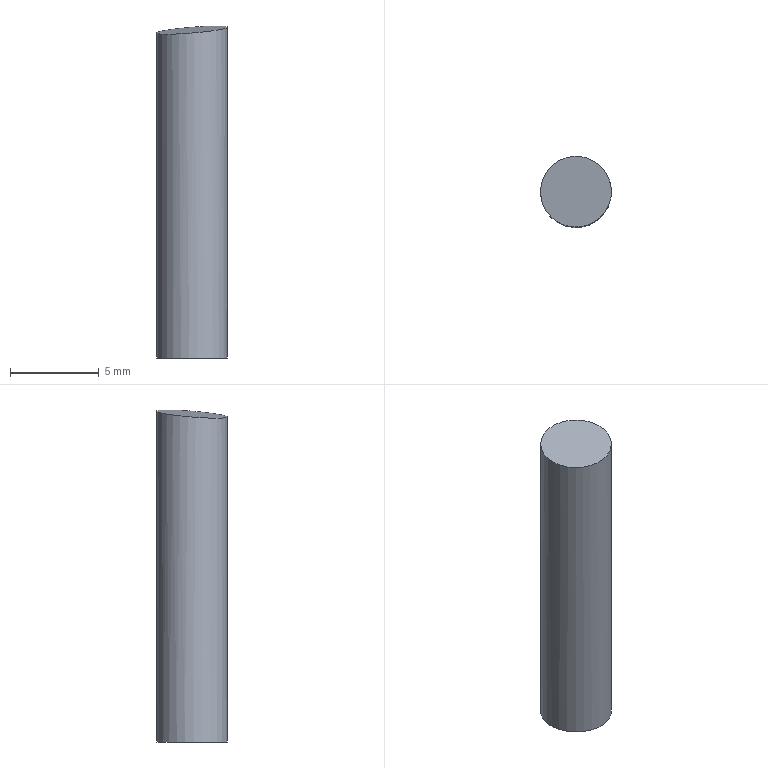Part | NX | features solid 2 | 1 solid | 3 faces | box 4 x 4 x 18.751 mm | volume 232.708 mm3 | plane 2 | cylinder 1 | commonest cylinder face diameters 4 x1
STEP:
#1=CARTESIAN_POINT('',(660.583,-7.761,-27.));
#2=VERTEX_POINT('',#1);
#3=CARTESIAN_POINT('',(658.583,-7.761,-27.));
#4=DIRECTION('',(0.,0.,1.));
#5=DIRECTION('',(1.,0.,0.));
#6=AXIS2_PLACEMENT_3D('',#3,#4,#5);
#7=CIRCLE('',#6,2.);
#8=EDGE_CURVE('',#2,#2,#7,.T.);
#9=ORIENTED_EDGE('',*,*,#8,.F.);
#10=EDGE_LOOP('',(#9));
#11=FACE_BOUND('',#10,.T.);
#12=CARTESIAN_POINT('',(658.583,-7.761,-27.));
#13=DIRECTION('',(0.,0.,-1.));
#14=DIRECTION('',(-1.,0.,0.));
#15=AXIS2_PLACEMENT_3D('',#12,#13,#14);
#16=PLANE('',#15);
#17=ADVANCED_FACE('',(#11),#16,.T.);
#18=CARTESIAN_POINT('',(657.162,-9.168,-8.714));
#19=VERTEX_POINT('',#18);
#20=CARTESIAN_POINT('',(658.583,-7.761,-8.482));
#21=DIRECTION('',(0.08207,0.08131,-0.9933));
#22=DIRECTION('',(-0.7057,-0.6991,-0.1155));
#23=AXIS2_PLACEMENT_3D('',#20,#21,#22);
#24=ELLIPSE('',#23,2.013,2.);
#25=EDGE_CURVE('',#19,#19,#24,.T.);
#26=ORIENTED_EDGE('',*,*,#25,.F.);
#27=EDGE_LOOP('',(#26));
#28=FACE_BOUND('',#27,.T.);
#29=CARTESIAN_POINT('',(770.198,-94.894,-6.392));
#30=DIRECTION('',(0.08207,0.08131,-0.9933));
#31=DIRECTION('',(0.9966,-0.01117,0.08143));
#32=AXIS2_PLACEMENT_3D('',#29,#30,#31);
#33=PLANE('',#32);
#34=ADVANCED_FACE('',(#28),#33,.F.);
#35=ORIENTED_EDGE('',*,*,#8,.T.);
#36=EDGE_LOOP('',(#35));
#37=FACE_BOUND('',#36,.T.);
#38=ORIENTED_EDGE('',*,*,#25,.T.);
#39=EDGE_LOOP('',(#38));
#40=FACE_BOUND('',#39,.T.);
#41=CARTESIAN_POINT('',(658.583,-7.761,-7.));
#42=DIRECTION('',(0.,0.,-1.));
#43=DIRECTION('',(-1.,0.,0.));
#44=AXIS2_PLACEMENT_3D('',#41,#42,#43);
#45=CYLINDRICAL_SURFACE('',#44,2.);
#46=ADVANCED_FACE('',(#37,#40),#45,.T.);
#47=CLOSED_SHELL('',(#17,#34,#46));
#48=MANIFOLD_SOLID_BREP('',#47);
#49=(LENGTH_UNIT()NAMED_UNIT(*)SI_UNIT(.MILLI.,.METRE.));
#50=UNCERTAINTY_MEASURE_WITH_UNIT(LENGTH_MEASURE(0.00001),#49,'','');
#51=(NAMED_UNIT(*)PLANE_ANGLE_UNIT()SI_UNIT($,.RADIAN.));
#52=(NAMED_UNIT(*)SI_UNIT($,.STERADIAN.)SOLID_ANGLE_UNIT());
#53=(GEOMETRIC_REPRESENTATION_CONTEXT(3)GLOBAL_UNCERTAINTY_ASSIGNED_CONTEXT((#50))GLOBAL_UNIT_ASSIGNED_CONTEXT((#49,#51,#52))REPRESENTATION_CONTEXT('',''));
#54=ADVANCED_BREP_SHAPE_REPRESENTATION('',(#48),#53);